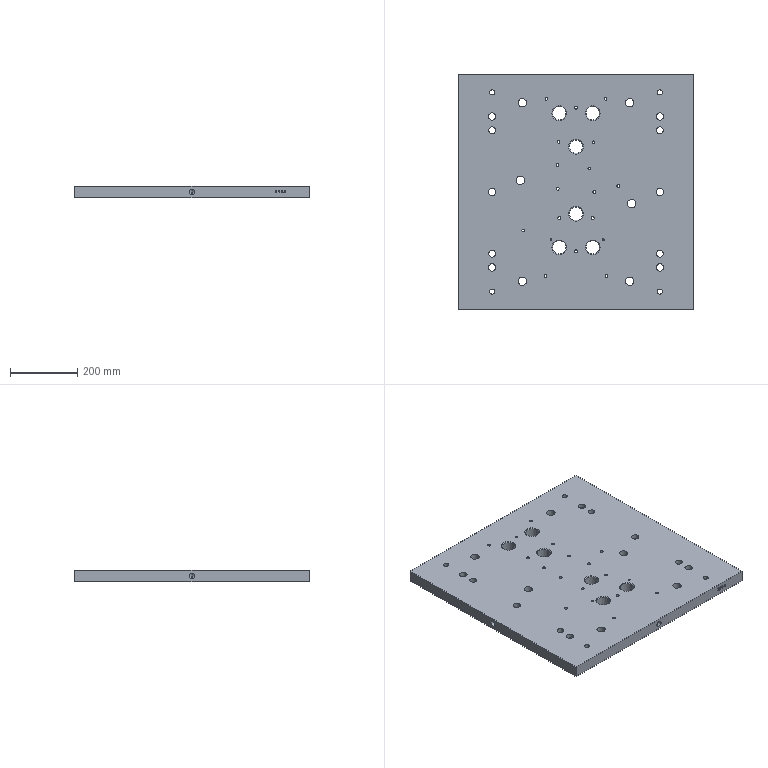Part | Creo | 1 solid | 317 faces | box 700 x 700 x 35 mm | volume 16458882 mm3 | cylinder 166 | plane 60 | other 59 | cone 32 | commonest cylinder face diameters 8.5 x28 14 x28 15 x12 22 x12 25 x12 31 x12